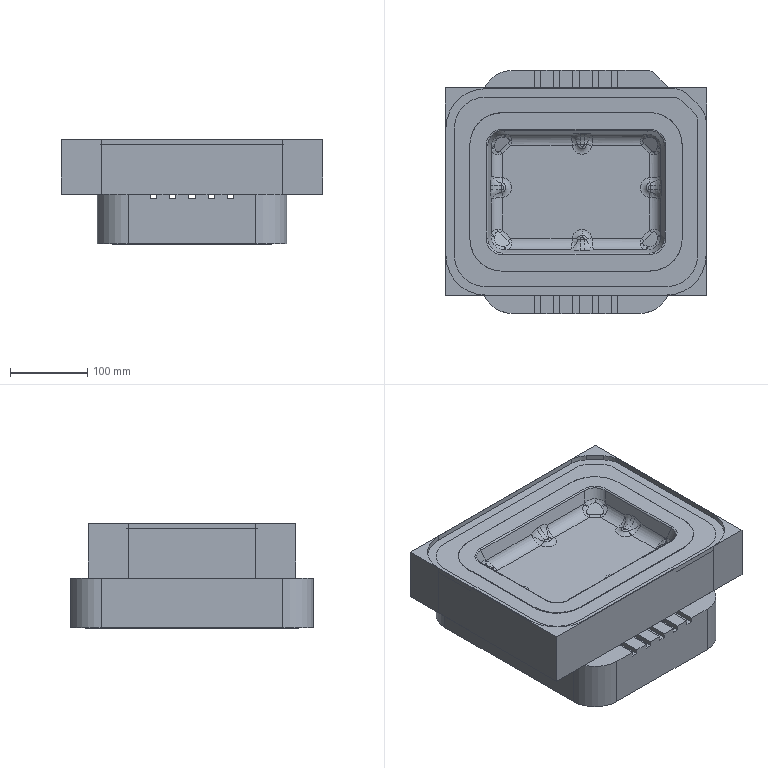Part | 4 solids | 655 faces | box 339.125 x 315.125 x 135.5 mm | volume 8727509 mm3 | plane 302 | cylinder 219 | spline 112 | torus 22 | commonest cylinder face diameters 2 x65 8 x65 16.88 x24 30.831 x24 80 x9 3.978 x8